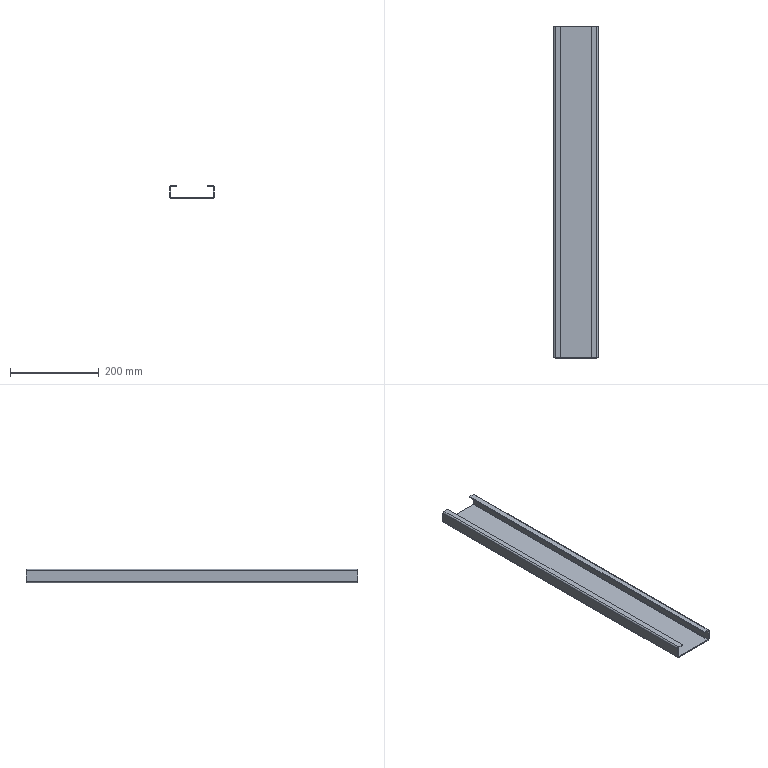Part | SolidWorks | features BaseBody 1 | 1 solid | 38 faces | box 100 x 750 x 30 mm | volume 331105 mm3 | plane 30 | cylinder 8 | commonest cylinder face diameters 1.473 x4 6.473 x4
STEP:
#1=CARTESIAN_POINT('',(35.,375.,25.));
#2=VERTEX_POINT('',#1);
#3=CARTESIAN_POINT('',(35.,-375.,25.));
#4=VERTEX_POINT('',#3);
#5=CARTESIAN_POINT('',(35.,-375.,25.));
#6=DIRECTION('',(0.,-1.,0.));
#7=VECTOR('',#6,1000.);
#8=LINE('',#5,#7);
#9=EDGE_CURVE('',#2,#4,#8,.T.);
#10=ORIENTED_EDGE('',*,*,#9,.T.);
#11=CARTESIAN_POINT('',(35.,-375.,27.5));
#12=VERTEX_POINT('',#11);
#13=CARTESIAN_POINT('',(35.,-375.,27.5));
#14=DIRECTION('',(0.,0.,-1.));
#15=VECTOR('',#14,1000.);
#16=LINE('',#13,#15);
#17=EDGE_CURVE('',#12,#4,#16,.T.);
#18=ORIENTED_EDGE('',*,*,#17,.F.);
#19=CARTESIAN_POINT('',(35.,375.,27.5));
#20=VERTEX_POINT('',#19);
#21=CARTESIAN_POINT('',(35.,0.,27.5));
#22=DIRECTION('',(0.,-1.,0.));
#23=VECTOR('',#22,1000.);
#24=LINE('',#21,#23);
#25=EDGE_CURVE('',#20,#12,#24,.T.);
#26=ORIENTED_EDGE('',*,*,#25,.F.);
#27=CARTESIAN_POINT('',(35.,375.,27.5));
#28=DIRECTION('',(0.,0.,-1.));
#29=VECTOR('',#28,1000.);
#30=LINE('',#27,#29);
#31=EDGE_CURVE('',#20,#2,#30,.T.);
#32=ORIENTED_EDGE('',*,*,#31,.T.);
#33=EDGE_LOOP('',(#10,#18,#26,#32));
#34=FACE_OUTER_BOUND('',#33,.T.);
#35=CARTESIAN_POINT('',(35.,-375.,27.5));
#36=DIRECTION('',(1.,0.,0.));
#37=DIRECTION('',(0.,0.,-1.));
#38=AXIS2_PLACEMENT_3D('',#35,#36,#37);
#39=PLANE('',#38);
#40=ADVANCED_FACE('',(#34),#39,.F.);
#41=CARTESIAN_POINT('',(46.763,375.,25.));
#42=VERTEX_POINT('',#41);
#43=CARTESIAN_POINT('',(35.,375.,25.));
#44=DIRECTION('',(-1.,0.,0.));
#45=VECTOR('',#44,1000.);
#46=LINE('',#43,#45);
#47=EDGE_CURVE('',#42,#2,#46,.T.);
#48=ORIENTED_EDGE('',*,*,#47,.F.);
#49=CARTESIAN_POINT('',(46.763,-375.,25.));
#50=VERTEX_POINT('',#49);
#51=CARTESIAN_POINT('',(46.763,-375.,25.));
#52=DIRECTION('',(0.,1.,0.));
#53=VECTOR('',#52,1000.);
#54=LINE('',#51,#53);
#55=EDGE_CURVE('',#50,#42,#54,.T.);
#56=ORIENTED_EDGE('',*,*,#55,.F.);
#57=CARTESIAN_POINT('',(47.5,-375.,25.));
#58=DIRECTION('',(1.,0.,0.));
#59=VECTOR('',#58,1000.);
#60=LINE('',#57,#59);
#61=EDGE_CURVE('',#4,#50,#60,.T.);
#62=ORIENTED_EDGE('',*,*,#61,.F.);
#63=ORIENTED_EDGE('',*,*,#9,.F.);
#64=EDGE_LOOP('',(#48,#56,#62,#63));
#65=FACE_OUTER_BOUND('',#64,.T.);
#66=CARTESIAN_POINT('',(0.,0.,25.));
#67=DIRECTION('',(0.,0.,-1.));
#68=DIRECTION('',(-1.,0.,0.));
#69=AXIS2_PLACEMENT_3D('',#66,#67,#68);
#70=PLANE('',#69);
#71=ADVANCED_FACE('',(#65),#70,.T.);
#72=CARTESIAN_POINT('',(46.763,375.,27.5));
#73=VERTEX_POINT('',#72);
#74=CARTESIAN_POINT('',(46.763,-375.,27.5));
#75=VERTEX_POINT('',#74);
#76=CARTESIAN_POINT('',(46.763,-375.,27.5));
#77=DIRECTION('',(0.,-1.,0.));
#78=VECTOR('',#77,1000.);
#79=LINE('',#76,#78);
#80=EDGE_CURVE('',#73,#75,#79,.T.);
#81=ORIENTED_EDGE('',*,*,#80,.F.);
#82=CARTESIAN_POINT('',(0.,375.,27.5));
#83=DIRECTION('',(-1.,0.,0.));
#84=VECTOR('',#83,1000.);
#85=LINE('',#82,#84);
#86=EDGE_CURVE('',#73,#20,#85,.T.);
#87=ORIENTED_EDGE('',*,*,#86,.T.);
#88=ORIENTED_EDGE('',*,*,#25,.T.);
#89=CARTESIAN_POINT('',(0.,-375.,27.5));
#90=DIRECTION('',(1.,0.,0.));
#91=VECTOR('',#90,1000.);
#92=LINE('',#89,#91);
#93=EDGE_CURVE('',#12,#75,#92,.T.);
#94=ORIENTED_EDGE('',*,*,#93,.T.);
#95=EDGE_LOOP('',(#81,#87,#88,#94));
#96=FACE_OUTER_BOUND('',#95,.T.);
#97=CARTESIAN_POINT('',(0.,0.,27.5));
#98=DIRECTION('',(0.,0.,-1.));
#99=DIRECTION('',(-1.,0.,0.));
#100=AXIS2_PLACEMENT_3D('',#97,#98,#99);
#101=PLANE('',#100);
#102=ADVANCED_FACE('',(#96),#101,.F.);
#103=CARTESIAN_POINT('',(46.763,-375.,27.5));
#104=DIRECTION('',(0.,0.,1.));
#105=VECTOR('',#104,1000.);
#106=LINE('',#103,#105);
#107=EDGE_CURVE('',#50,#75,#106,.T.);
#108=ORIENTED_EDGE('',*,*,#107,.T.);
#109=ORIENTED_EDGE('',*,*,#93,.F.);
#110=ORIENTED_EDGE('',*,*,#17,.T.);
#111=ORIENTED_EDGE('',*,*,#61,.T.);
#112=EDGE_LOOP('',(#108,#109,#110,#111));
#113=FACE_OUTER_BOUND('',#112,.T.);
#114=CARTESIAN_POINT('',(47.5,-375.,27.5));
#115=DIRECTION('',(0.,1.,0.));
#116=DIRECTION('',(0.,0.,-1.));
#117=AXIS2_PLACEMENT_3D('',#114,#115,#116);
#118=PLANE('',#117);
#119=ADVANCED_FACE('',(#113),#118,.F.);
#120=CARTESIAN_POINT('',(46.763,375.,25.));
#121=DIRECTION('',(0.,0.,1.));
#122=VECTOR('',#121,1000.);
#123=LINE('',#120,#122);
#124=EDGE_CURVE('',#42,#73,#123,.T.);
#125=ORIENTED_EDGE('',*,*,#124,.F.);
#126=ORIENTED_EDGE('',*,*,#47,.T.);
#127=ORIENTED_EDGE('',*,*,#31,.F.);
#128=ORIENTED_EDGE('',*,*,#86,.F.);
#129=EDGE_LOOP('',(#125,#126,#127,#128));
#130=FACE_OUTER_BOUND('',#129,.T.);
#131=CARTESIAN_POINT('',(35.,375.,27.5));
#132=DIRECTION('',(0.,-1.,0.));
#133=DIRECTION('',(-1.,0.,0.));
#134=AXIS2_PLACEMENT_3D('',#131,#132,#133);
#135=PLANE('',#134);
#136=ADVANCED_FACE('',(#130),#135,.F.);
#137=CARTESIAN_POINT('',(47.5,375.,24.263));
#138=VERTEX_POINT('',#137);
#139=CARTESIAN_POINT('',(47.5,-375.,24.263));
#140=VERTEX_POINT('',#139);
#141=CARTESIAN_POINT('',(47.5,375.,24.263));
#142=DIRECTION('',(0.,-1.,0.));
#143=VECTOR('',#142,1000.);
#144=LINE('',#141,#143);
#145=EDGE_CURVE('',#138,#140,#144,.T.);
#146=ORIENTED_EDGE('',*,*,#145,.T.);
#147=CARTESIAN_POINT('',(46.763,-375.,24.263));
#148=DIRECTION('',(0.,-1.,0.));
#149=DIRECTION('',(0.,0.,1.));
#150=AXIS2_PLACEMENT_3D('',#147,#148,#149);
#151=CIRCLE('',#150,0.7366);
#152=EDGE_CURVE('',#140,#50,#151,.T.);
#153=ORIENTED_EDGE('',*,*,#152,.T.);
#154=ORIENTED_EDGE('',*,*,#55,.T.);
#155=CARTESIAN_POINT('',(46.763,375.,24.263));
#156=DIRECTION('',(0.,1.,0.));
#157=DIRECTION('',(0.,0.,1.));
#158=AXIS2_PLACEMENT_3D('',#155,#156,#157);
#159=CIRCLE('',#158,0.7366);
#160=EDGE_CURVE('',#42,#138,#159,.T.);
#161=ORIENTED_EDGE('',*,*,#160,.T.);
#162=EDGE_LOOP('',(#146,#153,#154,#161));
#163=FACE_OUTER_BOUND('',#162,.T.);
#164=CARTESIAN_POINT('',(46.763,375.,24.263));
#165=DIRECTION('',(0.,1.,0.));
#166=DIRECTION('',(0.,0.,1.));
#167=AXIS2_PLACEMENT_3D('',#164,#165,#166);
#168=CYLINDRICAL_SURFACE('',#167,0.7366);
#169=ADVANCED_FACE('',(#163),#168,.F.);
#170=CARTESIAN_POINT('',(50.,375.,24.263));
#171=VERTEX_POINT('',#170);
#172=CARTESIAN_POINT('',(50.,-375.,24.263));
#173=VERTEX_POINT('',#172);
#174=CARTESIAN_POINT('',(50.,375.,24.263));
#175=DIRECTION('',(0.,-1.,0.));
#176=VECTOR('',#175,1000.);
#177=LINE('',#174,#176);
#178=EDGE_CURVE('',#171,#173,#177,.T.);
#179=ORIENTED_EDGE('',*,*,#178,.F.);
#180=CARTESIAN_POINT('',(46.763,375.,24.263));
#181=DIRECTION('',(0.,1.,0.));
#182=DIRECTION('',(0.,0.,1.));
#183=AXIS2_PLACEMENT_3D('',#180,#181,#182);
#184=CIRCLE('',#183,3.237);
#185=EDGE_CURVE('',#73,#171,#184,.T.);
#186=ORIENTED_EDGE('',*,*,#185,.F.);
#187=ORIENTED_EDGE('',*,*,#80,.T.);
#188=CARTESIAN_POINT('',(46.763,-375.,24.263));
#189=DIRECTION('',(0.,-1.,0.));
#190=DIRECTION('',(0.,0.,1.));
#191=AXIS2_PLACEMENT_3D('',#188,#189,#190);
#192=CIRCLE('',#191,3.237);
#193=EDGE_CURVE('',#173,#75,#192,.T.);
#194=ORIENTED_EDGE('',*,*,#193,.F.);
#195=EDGE_LOOP('',(#179,#186,#187,#194));
#196=FACE_OUTER_BOUND('',#195,.T.);
#197=CARTESIAN_POINT('',(46.763,375.,24.263));
#198=DIRECTION('',(0.,1.,0.));
#199=DIRECTION('',(0.,0.,1.));
#200=AXIS2_PLACEMENT_3D('',#197,#198,#199);
#201=CYLINDRICAL_SURFACE('',#200,3.237);
#202=ADVANCED_FACE('',(#196),#201,.T.);
#203=ORIENTED_EDGE('',*,*,#160,.F.);
#204=ORIENTED_EDGE('',*,*,#124,.T.);
#205=ORIENTED_EDGE('',*,*,#185,.T.);
#206=CARTESIAN_POINT('',(47.5,375.,24.263));
#207=DIRECTION('',(1.,0.,0.));
#208=VECTOR('',#207,1000.);
#209=LINE('',#206,#208);
#210=EDGE_CURVE('',#138,#171,#209,.T.);
#211=ORIENTED_EDGE('',*,*,#210,.F.);
#212=EDGE_LOOP('',(#203,#204,#205,#211));
#213=FACE_OUTER_BOUND('',#212,.T.);
#214=CARTESIAN_POINT('',(46.763,375.,24.263));
#215=DIRECTION('',(0.,-1.,0.));
#216=DIRECTION('',(0.,0.,-1.));
#217=AXIS2_PLACEMENT_3D('',#214,#215,#216);
#218=PLANE('',#217);
#219=ADVANCED_FACE('',(#213),#218,.F.);
#220=ORIENTED_EDGE('',*,*,#107,.F.);
#221=ORIENTED_EDGE('',*,*,#152,.F.);
#222=CARTESIAN_POINT('',(47.5,-375.,24.263));
#223=DIRECTION('',(1.,0.,0.));
#224=VECTOR('',#223,1000.);
#225=LINE('',#222,#224);
#226=EDGE_CURVE('',#140,#173,#225,.T.);
#227=ORIENTED_EDGE('',*,*,#226,.T.);
#228=ORIENTED_EDGE('',*,*,#193,.T.);
#229=EDGE_LOOP('',(#220,#221,#227,#228));
#230=FACE_OUTER_BOUND('',#229,.T.);
#231=CARTESIAN_POINT('',(46.763,-375.,24.263));
#232=DIRECTION('',(0.,-1.,0.));
#233=DIRECTION('',(0.,0.,-1.));
#234=AXIS2_PLACEMENT_3D('',#231,#232,#233);
#235=PLANE('',#234);
#236=ADVANCED_FACE('',(#230),#235,.T.);
#237=CARTESIAN_POINT('',(-35.,-375.,25.));
#238=VERTEX_POINT('',#237);
#239=CARTESIAN_POINT('',(-35.,375.,25.));
#240=VERTEX_POINT('',#239);
#241=CARTESIAN_POINT('',(-35.,375.,25.));
#242=DIRECTION('',(0.,1.,0.));
#243=VECTOR('',#242,1000.);
#244=LINE('',#241,#243);
#245=EDGE_CURVE('',#238,#240,#244,.T.);
#246=ORIENTED_EDGE('',*,*,#245,.T.);
#247=CARTESIAN_POINT('',(-35.,375.,27.5));
#248=VERTEX_POINT('',#247);
#249=CARTESIAN_POINT('',(-35.,375.,27.5));
#250=DIRECTION('',(0.,0.,-1.));
#251=VECTOR('',#250,1000.);
#252=LINE('',#249,#251);
#253=EDGE_CURVE('',#248,#240,#252,.T.);
#254=ORIENTED_EDGE('',*,*,#253,.F.);
#255=CARTESIAN_POINT('',(-35.,-375.,27.5));
#256=VERTEX_POINT('',#255);
#257=CARTESIAN_POINT('',(-35.,0.,27.5));
#258=DIRECTION('',(0.,1.,0.));
#259=VECTOR('',#258,1000.);
#260=LINE('',#257,#259);
#261=EDGE_CURVE('',#256,#248,#260,.T.);
#262=ORIENTED_EDGE('',*,*,#261,.F.);
#263=CARTESIAN_POINT('',(-35.,-375.,27.5));
#264=DIRECTION('',(0.,0.,-1.));
#265=VECTOR('',#264,1000.);
#266=LINE('',#263,#265);
#267=EDGE_CURVE('',#256,#238,#266,.T.);
#268=ORIENTED_EDGE('',*,*,#267,.T.);
#269=EDGE_LOOP('',(#246,#254,#262,#268));
#270=FACE_OUTER_BOUND('',#269,.T.);
#271=CARTESIAN_POINT('',(-35.,375.,27.5));
#272=DIRECTION('',(-1.,0.,0.));
#273=DIRECTION('',(0.,0.,1.));
#274=AXIS2_PLACEMENT_3D('',#271,#272,#273);
#275=PLANE('',#274);
#276=ADVANCED_FACE('',(#270),#275,.F.);
#277=CARTESIAN_POINT('',(-46.763,-375.,25.));
#278=VERTEX_POINT('',#277);
#279=CARTESIAN_POINT('',(-35.,-375.,25.));
#280=DIRECTION('',(1.,0.,0.));
#281=VECTOR('',#280,1000.);
#282=LINE('',#279,#281);
#283=EDGE_CURVE('',#278,#238,#282,.T.);
#284=ORIENTED_EDGE('',*,*,#283,.F.);
#285=CARTESIAN_POINT('',(-46.763,375.,25.));
#286=VERTEX_POINT('',#285);
#287=CARTESIAN_POINT('',(-46.763,375.,25.));
#288=DIRECTION('',(0.,-1.,0.));
#289=VECTOR('',#288,1000.);
#290=LINE('',#287,#289);
#291=EDGE_CURVE('',#286,#278,#290,.T.);
#292=ORIENTED_EDGE('',*,*,#291,.F.);
#293=CARTESIAN_POINT('',(-47.5,375.,25.));
#294=DIRECTION('',(-1.,0.,0.));
#295=VECTOR('',#294,1000.);
#296=LINE('',#293,#295);
#297=EDGE_CURVE('',#240,#286,#296,.T.);
#298=ORIENTED_EDGE('',*,*,#297,.F.);
#299=ORIENTED_EDGE('',*,*,#245,.F.);
#300=EDGE_LOOP('',(#284,#292,#298,#299));
#301=FACE_OUTER_BOUND('',#300,.T.);
#302=CARTESIAN_POINT('',(0.,0.,25.));
#303=DIRECTION('',(0.,0.,-1.));
#304=DIRECTION('',(0.,-1.,0.));
#305=AXIS2_PLACEMENT_3D('',#302,#303,#304);
#306=PLANE('',#305);
#307=ADVANCED_FACE('',(#301),#306,.T.);
#308=CARTESIAN_POINT('',(-46.763,-375.,27.5));
#309=VERTEX_POINT('',#308);
#310=CARTESIAN_POINT('',(-46.763,375.,27.5));
#311=VERTEX_POINT('',#310);
#312=CARTESIAN_POINT('',(-46.763,375.,27.5));
#313=DIRECTION('',(0.,1.,0.));
#314=VECTOR('',#313,1000.);
#315=LINE('',#312,#314);
#316=EDGE_CURVE('',#309,#311,#315,.T.);
#317=ORIENTED_EDGE('',*,*,#316,.F.);
#318=CARTESIAN_POINT('',(0.,-375.,27.5));
#319=DIRECTION('',(1.,0.,0.));
#320=VECTOR('',#319,1000.);
#321=LINE('',#318,#320);
#322=EDGE_CURVE('',#309,#256,#321,.T.);
#323=ORIENTED_EDGE('',*,*,#322,.T.);
#324=ORIENTED_EDGE('',*,*,#261,.T.);
#325=CARTESIAN_POINT('',(0.,375.,27.5));
#326=DIRECTION('',(-1.,0.,0.));
#327=VECTOR('',#326,1000.);
#328=LINE('',#325,#327);
#329=EDGE_CURVE('',#248,#311,#328,.T.);
#330=ORIENTED_EDGE('',*,*,#329,.T.);
#331=EDGE_LOOP('',(#317,#323,#324,#330));
#332=FACE_OUTER_BOUND('',#331,.T.);
#333=CARTESIAN_POINT('',(0.,0.,27.5));
#334=DIRECTION('',(0.,0.,-1.));
#335=DIRECTION('',(0.,-1.,0.));
#336=AXIS2_PLACEMENT_3D('',#333,#334,#335);
#337=PLANE('',#336);
#338=ADVANCED_FACE('',(#332),#337,.F.);
#339=CARTESIAN_POINT('',(-46.763,375.,27.5));
#340=DIRECTION('',(0.,0.,1.));
#341=VECTOR('',#340,1000.);
#342=LINE('',#339,#341);
#343=EDGE_CURVE('',#286,#311,#342,.T.);
#344=ORIENTED_EDGE('',*,*,#343,.T.);
#345=ORIENTED_EDGE('',*,*,#329,.F.);
#346=ORIENTED_EDGE('',*,*,#253,.T.);
#347=ORIENTED_EDGE('',*,*,#297,.T.);
#348=EDGE_LOOP('',(#344,#345,#346,#347));
#349=FACE_OUTER_BOUND('',#348,.T.);
#350=CARTESIAN_POINT('',(-47.5,375.,27.5));
#351=DIRECTION('',(0.,-1.,0.));
#352=DIRECTION('',(0.,0.,-1.));
#353=AXIS2_PLACEMENT_3D('',#350,#351,#352);
#354=PLANE('',#353);
#355=ADVANCED_FACE('',(#349),#354,.F.);
#356=CARTESIAN_POINT('',(-46.763,-375.,25.));
#357=DIRECTION('',(0.,0.,1.));
#358=VECTOR('',#357,1000.);
#359=LINE('',#356,#358);
#360=EDGE_CURVE('',#278,#309,#359,.T.);
#361=ORIENTED_EDGE('',*,*,#360,.F.);
#362=ORIENTED_EDGE('',*,*,#283,.T.);
#363=ORIENTED_EDGE('',*,*,#267,.F.);
#364=ORIENTED_EDGE('',*,*,#322,.F.);
#365=EDGE_LOOP('',(#361,#362,#363,#364));
#366=FACE_OUTER_BOUND('',#365,.T.);
#367=CARTESIAN_POINT('',(-35.,-375.,27.5));
#368=DIRECTION('',(0.,1.,0.));
#369=DIRECTION('',(0.,0.,-1.));
#370=AXIS2_PLACEMENT_3D('',#367,#368,#369);
#371=PLANE('',#370);
#372=ADVANCED_FACE('',(#366),#371,.F.);
#373=CARTESIAN_POINT('',(-47.5,-375.,24.263));
#374=VERTEX_POINT('',#373);
#375=CARTESIAN_POINT('',(-47.5,375.,24.263));
#376=VERTEX_POINT('',#375);
#377=CARTESIAN_POINT('',(-47.5,-375.,24.263));
#378=DIRECTION('',(0.,1.,0.));
#379=VECTOR('',#378,1000.);
#380=LINE('',#377,#379);
#381=EDGE_CURVE('',#374,#376,#380,.T.);
#382=ORIENTED_EDGE('',*,*,#381,.T.);
#383=CARTESIAN_POINT('',(-46.763,375.,24.263));
#384=DIRECTION('',(0.,1.,0.));
#385=DIRECTION('',(0.,0.,-1.));
#386=AXIS2_PLACEMENT_3D('',#383,#384,#385);
#387=CIRCLE('',#386,0.7366);
#388=EDGE_CURVE('',#376,#286,#387,.T.);
#389=ORIENTED_EDGE('',*,*,#388,.T.);
#390=ORIENTED_EDGE('',*,*,#291,.T.);
#391=CARTESIAN_POINT('',(-46.763,-375.,24.263));
#392=DIRECTION('',(0.,-1.,0.));
#393=DIRECTION('',(0.,0.,-1.));
#394=AXIS2_PLACEMENT_3D('',#391,#392,#393);
#395=CIRCLE('',#394,0.7366);
#396=EDGE_CURVE('',#278,#374,#395,.T.);
#397=ORIENTED_EDGE('',*,*,#396,.T.);
#398=EDGE_LOOP('',(#382,#389,#390,#397));
#399=FACE_OUTER_BOUND('',#398,.T.);
#400=CARTESIAN_POINT('',(-46.763,-375.,24.263));
#401=DIRECTION('',(0.,-1.,0.));
#402=DIRECTION('',(0.,0.,1.));
#403=AXIS2_PLACEMENT_3D('',#400,#401,#402);
#404=CYLINDRICAL_SURFACE('',#403,0.7366);
#405=ADVANCED_FACE('',(#399),#404,.F.);
#406=CARTESIAN_POINT('',(-50.,-375.,24.263));
#407=VERTEX_POINT('',#406);
#408=CARTESIAN_POINT('',(-50.,375.,24.263));
#409=VERTEX_POINT('',#408);
#410=CARTESIAN_POINT('',(-50.,-375.,24.263));
#411=DIRECTION('',(0.,1.,0.));
#412=VECTOR('',#411,1000.);
#413=LINE('',#410,#412);
#414=EDGE_CURVE('',#407,#409,#413,.T.);
#415=ORIENTED_EDGE('',*,*,#414,.F.);
#416=CARTESIAN_POINT('',(-46.763,-375.,24.263));
#417=DIRECTION('',(0.,-1.,0.));
#418=DIRECTION('',(0.,0.,-1.));
#419=AXIS2_PLACEMENT_3D('',#416,#417,#418);
#420=CIRCLE('',#419,3.237);
#421=EDGE_CURVE('',#309,#407,#420,.T.);
#422=ORIENTED_EDGE('',*,*,#421,.F.);
#423=ORIENTED_EDGE('',*,*,#316,.T.);
#424=CARTESIAN_POINT('',(-46.763,375.,24.263));
#425=DIRECTION('',(0.,1.,0.));
#426=DIRECTION('',(0.,0.,-1.));
#427=AXIS2_PLACEMENT_3D('',#424,#425,#426);
#428=CIRCLE('',#427,3.237);
#429=EDGE_CURVE('',#409,#311,#428,.T.);
#430=ORIENTED_EDGE('',*,*,#429,.F.);
#431=EDGE_LOOP('',(#415,#422,#423,#430));
#432=FACE_OUTER_BOUND('',#431,.T.);
#433=CARTESIAN_POINT('',(-46.763,-375.,24.263));
#434=DIRECTION('',(0.,-1.,0.));
#435=DIRECTION('',(0.,0.,1.));
#436=AXIS2_PLACEMENT_3D('',#433,#434,#435);
#437=CYLINDRICAL_SURFACE('',#436,3.237);
#438=ADVANCED_FACE('',(#432),#437,.T.);
#439=ORIENTED_EDGE('',*,*,#396,.F.);
#440=ORIENTED_EDGE('',*,*,#360,.T.);
#441=ORIENTED_EDGE('',*,*,#421,.T.);
#442=CARTESIAN_POINT('',(-47.5,-375.,24.263));
#443=DIRECTION('',(-1.,0.,0.));
#444=VECTOR('',#443,1000.);
#445=LINE('',#442,#444);
#446=EDGE_CURVE('',#374,#407,#445,.T.);
#447=ORIENTED_EDGE('',*,*,#446,.F.);
#448=EDGE_LOOP('',(#439,#440,#441,#447));
#449=FACE_OUTER_BOUND('',#448,.T.);
#450=CARTESIAN_POINT('',(-46.763,-375.,24.263));
#451=DIRECTION('',(0.,1.,0.));
#452=DIRECTION('',(1.,0.,0.));
#453=AXIS2_PLACEMENT_3D('',#450,#451,#452);
#454=PLANE('',#453);
#455=ADVANCED_FACE('',(#449),#454,.F.);
#456=ORIENTED_EDGE('',*,*,#343,.F.);
#457=ORIENTED_EDGE('',*,*,#388,.F.);
#458=CARTESIAN_POINT('',(-47.5,375.,24.263));
#459=DIRECTION('',(-1.,0.,0.));
#460=VECTOR('',#459,1000.);
#461=LINE('',#458,#460);
#462=EDGE_CURVE('',#376,#409,#461,.T.);
#463=ORIENTED_EDGE('',*,*,#462,.T.);
#464=ORIENTED_EDGE('',*,*,#429,.T.);
#465=EDGE_LOOP('',(#456,#457,#463,#464));
#466=FACE_OUTER_BOUND('',#465,.T.);
#467=CARTESIAN_POINT('',(-46.763,375.,24.263));
#468=DIRECTION('',(0.,1.,0.));
#469=DIRECTION('',(1.,0.,0.));
#470=AXIS2_PLACEMENT_3D('',#467,#468,#469);
#471=PLANE('',#470);
#472=ADVANCED_FACE('',(#466),#471,.T.);
#473=CARTESIAN_POINT('',(46.763,375.,0.));
#474=VERTEX_POINT('',#473);
#475=CARTESIAN_POINT('',(46.763,-375.,0.));
#476=VERTEX_POINT('',#475);
#477=CARTESIAN_POINT('',(46.763,375.,0.));
#478=DIRECTION('',(0.,-1.,0.));
#479=VECTOR('',#478,1000.);
#480=LINE('',#477,#479);
#481=EDGE_CURVE('',#474,#476,#480,.T.);
#482=ORIENTED_EDGE('',*,*,#481,.T.);
#483=CARTESIAN_POINT('',(47.5,-375.,0.7366));
#484=VERTEX_POINT('',#483);
#485=CARTESIAN_POINT('',(46.763,-375.,0.7366));
#486=DIRECTION('',(0.,-1.,0.));
#487=DIRECTION('',(0.,0.,1.));
#488=AXIS2_PLACEMENT_3D('',#485,#486,#487);
#489=CIRCLE('',#488,0.7366);
#490=EDGE_CURVE('',#476,#484,#489,.T.);
#491=ORIENTED_EDGE('',*,*,#490,.T.);
#492=CARTESIAN_POINT('',(47.5,375.,0.7366));
#493=VERTEX_POINT('',#492);
#494=CARTESIAN_POINT('',(47.5,-375.,0.7366));
#495=DIRECTION('',(0.,1.,0.));
#496=VECTOR('',#495,1000.);
#497=LINE('',#494,#496);
#498=EDGE_CURVE('',#484,#493,#497,.T.);
#499=ORIENTED_EDGE('',*,*,#498,.T.);
#500=CARTESIAN_POINT('',(46.763,375.,0.7366));
#501=DIRECTION('',(0.,1.,0.));
#502=DIRECTION('',(0.,0.,1.));
#503=AXIS2_PLACEMENT_3D('',#500,#501,#502);
#504=CIRCLE('',#503,0.7366);
#505=EDGE_CURVE('',#493,#474,#504,.T.);
#506=ORIENTED_EDGE('',*,*,#505,.T.);
#507=EDGE_LOOP('',(#482,#491,#499,#506));
#508=FACE_OUTER_BOUND('',#507,.T.);
#509=CARTESIAN_POINT('',(46.763,375.,0.7366));
#510=DIRECTION('',(0.,1.,0.));
#511=DIRECTION('',(1.,0.,0.));
#512=AXIS2_PLACEMENT_3D('',#509,#510,#511);
#513=CYLINDRICAL_SURFACE('',#512,0.7366);
#514=ADVANCED_FACE('',(#508),#513,.F.);
#515=CARTESIAN_POINT('',(46.763,375.,-2.5));
#516=VERTEX_POINT('',#515);
#517=CARTESIAN_POINT('',(46.763,-375.,-2.5));
#518=VERTEX_POINT('',#517);
#519=CARTESIAN_POINT('',(46.763,375.,-2.5));
#520=DIRECTION('',(0.,-1.,0.));
#521=VECTOR('',#520,1000.);
#522=LINE('',#519,#521);
#523=EDGE_CURVE('',#516,#518,#522,.T.);
#524=ORIENTED_EDGE('',*,*,#523,.F.);
#525=CARTESIAN_POINT('',(50.,375.,0.7366));
#526=VERTEX_POINT('',#525);
#527=CARTESIAN_POINT('',(46.763,375.,0.7366));
#528=DIRECTION('',(0.,1.,0.));
#529=DIRECTION('',(0.,0.,1.));
#530=AXIS2_PLACEMENT_3D('',#527,#528,#529);
#531=CIRCLE('',#530,3.237);
#532=EDGE_CURVE('',#526,#516,#531,.T.);
#533=ORIENTED_EDGE('',*,*,#532,.F.);
#534=CARTESIAN_POINT('',(50.,-375.,0.7366));
#535=VERTEX_POINT('',#534);
#536=CARTESIAN_POINT('',(50.,-375.,0.7366));
#537=DIRECTION('',(0.,-1.,0.));
#538=VECTOR('',#537,1000.);
#539=LINE('',#536,#538);
#540=EDGE_CURVE('',#526,#535,#539,.T.);
#541=ORIENTED_EDGE('',*,*,#540,.T.);
#542=CARTESIAN_POINT('',(46.763,-375.,0.7366));
#543=DIRECTION('',(0.,-1.,0.));
#544=DIRECTION('',(0.,0.,1.));
#545=AXIS2_PLACEMENT_3D('',#542,#543,#544);
#546=CIRCLE('',#545,3.237);
#547=EDGE_CURVE('',#518,#535,#546,.T.);
#548=ORIENTED_EDGE('',*,*,#547,.F.);
#549=EDGE_LOOP('',(#524,#533,#541,#548));
#550=FACE_OUTER_BOUND('',#549,.T.);
#551=CARTESIAN_POINT('',(46.763,375.,0.7366));
#552=DIRECTION('',(0.,1.,0.));
#553=DIRECTION('',(1.,0.,0.));
#554=AXIS2_PLACEMENT_3D('',#551,#552,#553);
#555=CYLINDRICAL_SURFACE('',#554,3.237);
#556=ADVANCED_FACE('',(#550),#555,.T.);
#557=ORIENTED_EDGE('',*,*,#505,.F.);
#558=CARTESIAN_POINT('',(47.5,375.,0.7366));
#559=DIRECTION('',(1.,0.,0.));
#560=VECTOR('',#559,1000.);
#561=LINE('',#558,#560);
#562=EDGE_CURVE('',#493,#526,#561,.T.);
#563=ORIENTED_EDGE('',*,*,#562,.T.);
#564=ORIENTED_EDGE('',*,*,#532,.T.);
#565=CARTESIAN_POINT('',(46.763,375.,0.));
#566=DIRECTION('',(0.,0.,-1.));
#567=VECTOR('',#566,1000.);
#568=LINE('',#565,#567);
#569=EDGE_CURVE('',#474,#516,#568,.T.);
#570=ORIENTED_EDGE('',*,*,#569,.F.);
#571=EDGE_LOOP('',(#557,#563,#564,#570));
#572=FACE_OUTER_BOUND('',#571,.T.);
#573=CARTESIAN_POINT('',(46.763,375.,0.7366));
#574=DIRECTION('',(0.,-1.,0.));
#575=DIRECTION('',(0.,0.,-1.));
#576=AXIS2_PLACEMENT_3D('',#573,#574,#575);
#577=PLANE('',#576);
#578=ADVANCED_FACE('',(#572),#577,.F.);
#579=CARTESIAN_POINT('',(50.,-375.,0.7366));
#580=DIRECTION('',(1.,0.,0.));
#581=VECTOR('',#580,1000.);
#582=LINE('',#579,#581);
#583=EDGE_CURVE('',#484,#535,#582,.T.);
#584=ORIENTED_EDGE('',*,*,#583,.F.);
#585=ORIENTED_EDGE('',*,*,#490,.F.);
#586=CARTESIAN_POINT('',(46.763,-375.,0.));
#587=DIRECTION('',(0.,0.,-1.));
#588=VECTOR('',#587,1000.);
#589=LINE('',#586,#588);
#590=EDGE_CURVE('',#476,#518,#589,.T.);
#591=ORIENTED_EDGE('',*,*,#590,.T.);
#592=ORIENTED_EDGE('',*,*,#547,.T.);
#593=EDGE_LOOP('',(#584,#585,#591,#592));
#594=FACE_OUTER_BOUND('',#593,.T.);
#595=CARTESIAN_POINT('',(46.763,-375.,0.7366));
#596=DIRECTION('',(0.,-1.,0.));
#597=DIRECTION('',(0.,0.,-1.));
#598=AXIS2_PLACEMENT_3D('',#595,#596,#597);
#599=PLANE('',#598);
#600=ADVANCED_FACE('',(#594),#599,.T.);
#601=CARTESIAN_POINT('',(-46.763,-375.,0.));
#602=VERTEX_POINT('',#601);
#603=CARTESIAN_POINT('',(-46.763,375.,0.));
#604=VERTEX_POINT('',#603);
#605=CARTESIAN_POINT('',(-46.763,-375.,0.));
#606=DIRECTION('',(0.,1.,0.));
#607=VECTOR('',#606,1000.);
#608=LINE('',#605,#607);
#609=EDGE_CURVE('',#602,#604,#608,.T.);
#610=ORIENTED_EDGE('',*,*,#609,.T.);
#611=CARTESIAN_POINT('',(-47.5,375.,0.7366));
#612=VERTEX_POINT('',#611);
#613=CARTESIAN_POINT('',(-46.763,375.,0.7366));
#614=DIRECTION('',(0.,1.,0.));
#615=DIRECTION('',(0.,0.,-1.));
#616=AXIS2_PLACEMENT_3D('',#613,#614,#615);
#617=CIRCLE('',#616,0.7366);
#618=EDGE_CURVE('',#604,#612,#617,.T.);
#619=ORIENTED_EDGE('',*,*,#618,.T.);
#620=CARTESIAN_POINT('',(-47.5,-375.,0.7366));
#621=VERTEX_POINT('',#620);
#622=CARTESIAN_POINT('',(-47.5,375.,0.7366));
#623=DIRECTION('',(0.,-1.,0.));
#624=VECTOR('',#623,1000.);
#625=LINE('',#622,#624);
#626=EDGE_CURVE('',#612,#621,#625,.T.);
#627=ORIENTED_EDGE('',*,*,#626,.T.);
#628=CARTESIAN_POINT('',(-46.763,-375.,0.7366));
#629=DIRECTION('',(0.,-1.,0.));
#630=DIRECTION('',(0.,0.,-1.));
#631=AXIS2_PLACEMENT_3D('',#628,#629,#630);
#632=CIRCLE('',#631,0.7366);
#633=EDGE_CURVE('',#621,#602,#632,.T.);
#634=ORIENTED_EDGE('',*,*,#633,.T.);
#635=EDGE_LOOP('',(#610,#619,#627,#634));
#636=FACE_OUTER_BOUND('',#635,.T.);
#637=CARTESIAN_POINT('',(-46.763,-375.,0.7366));
#638=DIRECTION('',(0.,-1.,0.));
#639=DIRECTION('',(-1.,0.,0.));
#640=AXIS2_PLACEMENT_3D('',#637,#638,#639);
#641=CYLINDRICAL_SURFACE('',#640,0.7366);
#642=ADVANCED_FACE('',(#636),#641,.F.);
#643=CARTESIAN_POINT('',(-46.763,-375.,-2.5));
#644=VERTEX_POINT('',#643);
#645=CARTESIAN_POINT('',(-46.763,375.,-2.5));
#646=VERTEX_POINT('',#645);
#647=CARTESIAN_POINT('',(-46.763,-375.,-2.5));
#648=DIRECTION('',(0.,1.,0.));
#649=VECTOR('',#648,1000.);
#650=LINE('',#647,#649);
#651=EDGE_CURVE('',#644,#646,#650,.T.);
#652=ORIENTED_EDGE('',*,*,#651,.F.);
#653=CARTESIAN_POINT('',(-50.,-375.,0.7366));
#654=VERTEX_POINT('',#653);
#655=CARTESIAN_POINT('',(-46.763,-375.,0.7366));
#656=DIRECTION('',(0.,-1.,0.));
#657=DIRECTION('',(0.,0.,-1.));
#658=AXIS2_PLACEMENT_3D('',#655,#656,#657);
#659=CIRCLE('',#658,3.237);
#660=EDGE_CURVE('',#654,#644,#659,.T.);
#661=ORIENTED_EDGE('',*,*,#660,.F.);
#662=CARTESIAN_POINT('',(-50.,375.,0.7366));
#663=VERTEX_POINT('',#662);
#664=CARTESIAN_POINT('',(-50.,375.,0.7366));
#665=DIRECTION('',(0.,1.,0.));
#666=VECTOR('',#665,1000.);
#667=LINE('',#664,#666);
#668=EDGE_CURVE('',#654,#663,#667,.T.);
#669=ORIENTED_EDGE('',*,*,#668,.T.);
#670=CARTESIAN_POINT('',(-46.763,375.,0.7366));
#671=DIRECTION('',(0.,1.,0.));
#672=DIRECTION('',(0.,0.,-1.));
#673=AXIS2_PLACEMENT_3D('',#670,#671,#672);
#674=CIRCLE('',#673,3.237);
#675=EDGE_CURVE('',#646,#663,#674,.T.);
#676=ORIENTED_EDGE('',*,*,#675,.F.);
#677=EDGE_LOOP('',(#652,#661,#669,#676));
#678=FACE_OUTER_BOUND('',#677,.T.);
#679=CARTESIAN_POINT('',(-46.763,-375.,0.7366));
#680=DIRECTION('',(0.,-1.,0.));
#681=DIRECTION('',(-1.,0.,0.));
#682=AXIS2_PLACEMENT_3D('',#679,#680,#681);
#683=CYLINDRICAL_SURFACE('',#682,3.237);
#684=ADVANCED_FACE('',(#678),#683,.T.);
#685=ORIENTED_EDGE('',*,*,#633,.F.);
#686=CARTESIAN_POINT('',(-47.5,-375.,0.7366));
#687=DIRECTION('',(-1.,0.,0.));
#688=VECTOR('',#687,1000.);
#689=LINE('',#686,#688);
#690=EDGE_CURVE('',#621,#654,#689,.T.);
#691=ORIENTED_EDGE('',*,*,#690,.T.);
#692=ORIENTED_EDGE('',*,*,#660,.T.);
#693=CARTESIAN_POINT('',(-46.763,-375.,0.));
#694=DIRECTION('',(0.,0.,-1.));
#695=VECTOR('',#694,1000.);
#696=LINE('',#693,#695);
#697=EDGE_CURVE('',#602,#644,#696,.T.);
#698=ORIENTED_EDGE('',*,*,#697,.F.);
#699=EDGE_LOOP('',(#685,#691,#692,#698));
#700=FACE_OUTER_BOUND('',#699,.T.);
#701=CARTESIAN_POINT('',(-46.763,-375.,0.7366));
#702=DIRECTION('',(0.,1.,0.));
#703=DIRECTION('',(0.,0.,-1.));
#704=AXIS2_PLACEMENT_3D('',#701,#702,#703);
#705=PLANE('',#704);
#706=ADVANCED_FACE('',(#700),#705,.F.);
#707=CARTESIAN_POINT('',(-50.,375.,0.7366));
#708=DIRECTION('',(-1.,0.,0.));
#709=VECTOR('',#708,1000.);
#710=LINE('',#707,#709);
#711=EDGE_CURVE('',#612,#663,#710,.T.);
#712=ORIENTED_EDGE('',*,*,#711,.F.);
#713=ORIENTED_EDGE('',*,*,#618,.F.);
#714=CARTESIAN_POINT('',(-46.763,375.,0.));
#715=DIRECTION('',(0.,0.,-1.));
#716=VECTOR('',#715,1000.);
#717=LINE('',#714,#716);
#718=EDGE_CURVE('',#604,#646,#717,.T.);
#719=ORIENTED_EDGE('',*,*,#718,.T.);
#720=ORIENTED_EDGE('',*,*,#675,.T.);
#721=EDGE_LOOP('',(#712,#713,#719,#720));
#722=FACE_OUTER_BOUND('',#721,.T.);
#723=CARTESIAN_POINT('',(-46.763,375.,0.7366));
#724=DIRECTION('',(0.,1.,0.));
#725=DIRECTION('',(0.,0.,-1.));
#726=AXIS2_PLACEMENT_3D('',#723,#724,#725);
#727=PLANE('',#726);
#728=ADVANCED_FACE('',(#722),#727,.T.);
#729=ORIENTED_EDGE('',*,*,#590,.F.);
#730=CARTESIAN_POINT('',(50.,-375.,0.));
#731=DIRECTION('',(1.,0.,0.));
#732=VECTOR('',#731,1000.);
#733=LINE('',#730,#732);
#734=EDGE_CURVE('',#602,#476,#733,.T.);
#735=ORIENTED_EDGE('',*,*,#734,.F.);
#736=ORIENTED_EDGE('',*,*,#697,.T.);
#737=CARTESIAN_POINT('',(50.,-375.,-2.5));
#738=DIRECTION('',(1.,0.,0.));
#739=VECTOR('',#738,1000.);
#740=LINE('',#737,#739);
#741=EDGE_CURVE('',#644,#518,#740,.T.);
#742=ORIENTED_EDGE('',*,*,#741,.T.);
#743=EDGE_LOOP('',(#729,#735,#736,#742));
#744=FACE_OUTER_BOUND('',#743,.T.);
#745=CARTESIAN_POINT('',(50.,-375.,-2.5));
#746=DIRECTION('',(0.,-1.,0.));
#747=DIRECTION('',(0.,0.,-1.));
#748=AXIS2_PLACEMENT_3D('',#745,#746,#747);
#749=PLANE('',#748);
#750=ADVANCED_FACE('',(#744),#749,.T.);
#751=CARTESIAN_POINT('',(50.,375.,0.));
#752=DIRECTION('',(-1.,0.,0.));
#753=VECTOR('',#752,1000.);
#754=LINE('',#751,#753);
#755=EDGE_CURVE('',#474,#604,#754,.T.);
#756=ORIENTED_EDGE('',*,*,#755,.F.);
#757=ORIENTED_EDGE('',*,*,#569,.T.);
#758=CARTESIAN_POINT('',(50.,375.,-2.5));
#759=DIRECTION('',(-1.,0.,0.));
#760=VECTOR('',#759,1000.);
#761=LINE('',#758,#760);
#762=EDGE_CURVE('',#516,#646,#761,.T.);
#763=ORIENTED_EDGE('',*,*,#762,.T.);
#764=ORIENTED_EDGE('',*,*,#718,.F.);
#765=EDGE_LOOP('',(#756,#757,#763,#764));
#766=FACE_OUTER_BOUND('',#765,.T.);
#767=CARTESIAN_POINT('',(50.,375.,-2.5));
#768=DIRECTION('',(0.,1.,0.));
#769=DIRECTION('',(1.,0.,0.));
#770=AXIS2_PLACEMENT_3D('',#767,#768,#769);
#771=PLANE('',#770);
#772=ADVANCED_FACE('',(#766),#771,.T.);
#773=ORIENTED_EDGE('',*,*,#481,.F.);
#774=ORIENTED_EDGE('',*,*,#755,.T.);
#775=ORIENTED_EDGE('',*,*,#609,.F.);
#776=ORIENTED_EDGE('',*,*,#734,.T.);
#777=EDGE_LOOP('',(#773,#774,#775,#776));
#778=FACE_OUTER_BOUND('',#777,.T.);
#779=CARTESIAN_POINT('',(0.,0.,0.));
#780=DIRECTION('',(0.,0.,-1.));
#781=DIRECTION('',(0.,-1.,0.));
#782=AXIS2_PLACEMENT_3D('',#779,#780,#781);
#783=PLANE('',#782);
#784=ADVANCED_FACE('',(#778),#783,.F.);
#785=ORIENTED_EDGE('',*,*,#762,.F.);
#786=ORIENTED_EDGE('',*,*,#523,.T.);
#787=ORIENTED_EDGE('',*,*,#741,.F.);
#788=ORIENTED_EDGE('',*,*,#651,.T.);
#789=EDGE_LOOP('',(#785,#786,#787,#788));
#790=FACE_OUTER_BOUND('',#789,.T.);
#791=CARTESIAN_POINT('',(0.,0.,-2.5));
#792=DIRECTION('',(0.,0.,-1.));
#793=DIRECTION('',(0.,-1.,0.));
#794=AXIS2_PLACEMENT_3D('',#791,#792,#793);
#795=PLANE('',#794);
#796=ADVANCED_FACE('',(#790),#795,.T.);
#797=CARTESIAN_POINT('',(-47.5,375.,0.));
#798=DIRECTION('',(0.,0.,-1.));
#799=VECTOR('',#798,1000.);
#800=LINE('',#797,#799);
#801=EDGE_CURVE('',#376,#612,#800,.T.);
#802=ORIENTED_EDGE('',*,*,#801,.F.);
#803=ORIENTED_EDGE('',*,*,#381,.F.);
#804=CARTESIAN_POINT('',(-47.5,-375.,27.5));
#805=DIRECTION('',(0.,0.,1.));
#806=VECTOR('',#805,1000.);
#807=LINE('',#804,#806);
#808=EDGE_CURVE('',#621,#374,#807,.T.);
#809=ORIENTED_EDGE('',*,*,#808,.F.);
#810=ORIENTED_EDGE('',*,*,#626,.F.);
#811=EDGE_LOOP('',(#802,#803,#809,#810));
#812=FACE_OUTER_BOUND('',#811,.T.);
#813=CARTESIAN_POINT('',(-47.5,0.,0.));
#814=DIRECTION('',(1.,0.,0.));
#815=DIRECTION('',(0.,0.,1.));
#816=AXIS2_PLACEMENT_3D('',#813,#814,#815);
#817=PLANE('',#816);
#818=ADVANCED_FACE('',(#812),#817,.T.);
#819=ORIENTED_EDGE('',*,*,#414,.T.);
#820=CARTESIAN_POINT('',(-50.,375.,0.));
#821=DIRECTION('',(0.,0.,-1.));
#822=VECTOR('',#821,1000.);
#823=LINE('',#820,#822);
#824=EDGE_CURVE('',#409,#663,#823,.T.);
#825=ORIENTED_EDGE('',*,*,#824,.T.);
#826=ORIENTED_EDGE('',*,*,#668,.F.);
#827=CARTESIAN_POINT('',(-50.,-375.,0.));
#828=DIRECTION('',(0.,0.,1.));
#829=VECTOR('',#828,1000.);
#830=LINE('',#827,#829);
#831=EDGE_CURVE('',#654,#407,#830,.T.);
#832=ORIENTED_EDGE('',*,*,#831,.T.);
#833=EDGE_LOOP('',(#819,#825,#826,#832));
#834=FACE_OUTER_BOUND('',#833,.T.);
#835=CARTESIAN_POINT('',(-50.,0.,0.));
#836=DIRECTION('',(1.,0.,0.));
#837=DIRECTION('',(0.,0.,1.));
#838=AXIS2_PLACEMENT_3D('',#835,#836,#837);
#839=PLANE('',#838);
#840=ADVANCED_FACE('',(#834),#839,.F.);
#841=ORIENTED_EDGE('',*,*,#446,.T.);
#842=ORIENTED_EDGE('',*,*,#831,.F.);
#843=ORIENTED_EDGE('',*,*,#690,.F.);
#844=ORIENTED_EDGE('',*,*,#808,.T.);
#845=EDGE_LOOP('',(#841,#842,#843,#844));
#846=FACE_OUTER_BOUND('',#845,.T.);
#847=CARTESIAN_POINT('',(-50.,-375.,27.5));
#848=DIRECTION('',(0.,1.,0.));
#849=DIRECTION('',(1.,0.,0.));
#850=AXIS2_PLACEMENT_3D('',#847,#848,#849);
#851=PLANE('',#850);
#852=ADVANCED_FACE('',(#846),#851,.F.);
#853=ORIENTED_EDGE('',*,*,#462,.F.);
#854=ORIENTED_EDGE('',*,*,#801,.T.);
#855=ORIENTED_EDGE('',*,*,#711,.T.);
#856=ORIENTED_EDGE('',*,*,#824,.F.);
#857=EDGE_LOOP('',(#853,#854,#855,#856));
#858=FACE_OUTER_BOUND('',#857,.T.);
#859=CARTESIAN_POINT('',(-50.,375.,0.));
#860=DIRECTION('',(0.,-1.,0.));
#861=DIRECTION('',(0.,0.,-1.));
#862=AXIS2_PLACEMENT_3D('',#859,#860,#861);
#863=PLANE('',#862);
#864=ADVANCED_FACE('',(#858),#863,.F.);
#865=CARTESIAN_POINT('',(47.5,-375.,0.));
#866=DIRECTION('',(0.,0.,-1.));
#867=VECTOR('',#866,1000.);
#868=LINE('',#865,#867);
#869=EDGE_CURVE('',#140,#484,#868,.T.);
#870=ORIENTED_EDGE('',*,*,#869,.F.);
#871=ORIENTED_EDGE('',*,*,#145,.F.);
#872=CARTESIAN_POINT('',(47.5,375.,27.5));
#873=DIRECTION('',(0.,0.,1.));
#874=VECTOR('',#873,1000.);
#875=LINE('',#872,#874);
#876=EDGE_CURVE('',#493,#138,#875,.T.);
#877=ORIENTED_EDGE('',*,*,#876,.F.);
#878=ORIENTED_EDGE('',*,*,#498,.F.);
#879=EDGE_LOOP('',(#870,#871,#877,#878));
#880=FACE_OUTER_BOUND('',#879,.T.);
#881=CARTESIAN_POINT('',(47.5,0.,0.));
#882=DIRECTION('',(-1.,0.,0.));
#883=DIRECTION('',(0.,1.,0.));
#884=AXIS2_PLACEMENT_3D('',#881,#882,#883);
#885=PLANE('',#884);
#886=ADVANCED_FACE('',(#880),#885,.T.);
#887=ORIENTED_EDGE('',*,*,#178,.T.);
#888=CARTESIAN_POINT('',(50.,-375.,0.));
#889=DIRECTION('',(0.,0.,-1.));
#890=VECTOR('',#889,1000.);
#891=LINE('',#888,#890);
#892=EDGE_CURVE('',#173,#535,#891,.T.);
#893=ORIENTED_EDGE('',*,*,#892,.T.);
#894=ORIENTED_EDGE('',*,*,#540,.F.);
#895=CARTESIAN_POINT('',(50.,375.,0.));
#896=DIRECTION('',(0.,0.,1.));
#897=VECTOR('',#896,1000.);
#898=LINE('',#895,#897);
#899=EDGE_CURVE('',#526,#171,#898,.T.);
#900=ORIENTED_EDGE('',*,*,#899,.T.);
#901=EDGE_LOOP('',(#887,#893,#894,#900));
#902=FACE_OUTER_BOUND('',#901,.T.);
#903=CARTESIAN_POINT('',(50.,0.,0.));
#904=DIRECTION('',(-1.,0.,0.));
#905=DIRECTION('',(0.,1.,0.));
#906=AXIS2_PLACEMENT_3D('',#903,#904,#905);
#907=PLANE('',#906);
#908=ADVANCED_FACE('',(#902),#907,.F.);
#909=ORIENTED_EDGE('',*,*,#210,.T.);
#910=ORIENTED_EDGE('',*,*,#899,.F.);
#911=ORIENTED_EDGE('',*,*,#562,.F.);
#912=ORIENTED_EDGE('',*,*,#876,.T.);
#913=EDGE_LOOP('',(#909,#910,#911,#912));
#914=FACE_OUTER_BOUND('',#913,.T.);
#915=CARTESIAN_POINT('',(50.,375.,27.5));
#916=DIRECTION('',(0.,-1.,0.));
#917=DIRECTION('',(0.,0.,-1.));
#918=AXIS2_PLACEMENT_3D('',#915,#916,#917);
#919=PLANE('',#918);
#920=ADVANCED_FACE('',(#914),#919,.F.);
#921=ORIENTED_EDGE('',*,*,#226,.F.);
#922=ORIENTED_EDGE('',*,*,#869,.T.);
#923=ORIENTED_EDGE('',*,*,#583,.T.);
#924=ORIENTED_EDGE('',*,*,#892,.F.);
#925=EDGE_LOOP('',(#921,#922,#923,#924));
#926=FACE_OUTER_BOUND('',#925,.T.);
#927=CARTESIAN_POINT('',(50.,-375.,0.));
#928=DIRECTION('',(0.,1.,0.));
#929=DIRECTION('',(1.,0.,0.));
#930=AXIS2_PLACEMENT_3D('',#927,#928,#929);
#931=PLANE('',#930);
#932=ADVANCED_FACE('',(#926),#931,.F.);
#933=CLOSED_SHELL('',(#40,#71,#102,#119,#136,#169,#202,#219,#236,#276,#307,#338,#355,#372,#405,#438,#455,#472,#514,#556,#578,#600,#642,#684,#706,#728,#750,#772,#784,#796,#818,#840,#852,#864,#886,#908,#920,#932));
#934=MANIFOLD_SOLID_BREP('',#933);
#935=CARTESIAN_POINT('',(0.,0.,0.));
#936=DIRECTION('',(0.,0.,1.));
#937=DIRECTION('',(1.,0.,0.));
#938=AXIS2_PLACEMENT_3D('',#935,#936,#937);
#939=(LENGTH_UNIT()NAMED_UNIT(*)SI_UNIT(.MILLI.,.METRE.));
#940=UNCERTAINTY_MEASURE_WITH_UNIT(LENGTH_MEASURE(0.00001),#939,'','');
#941=(NAMED_UNIT(*)PLANE_ANGLE_UNIT()SI_UNIT($,.RADIAN.));
#942=(NAMED_UNIT(*)SI_UNIT($,.STERADIAN.)SOLID_ANGLE_UNIT());
#943=(GEOMETRIC_REPRESENTATION_CONTEXT(3)GLOBAL_UNCERTAINTY_ASSIGNED_CONTEXT((#940))GLOBAL_UNIT_ASSIGNED_CONTEXT((#939,#941,#942))REPRESENTATION_CONTEXT('',''));
#944=ADVANCED_BREP_SHAPE_REPRESENTATION('',(#934,#938),#943);